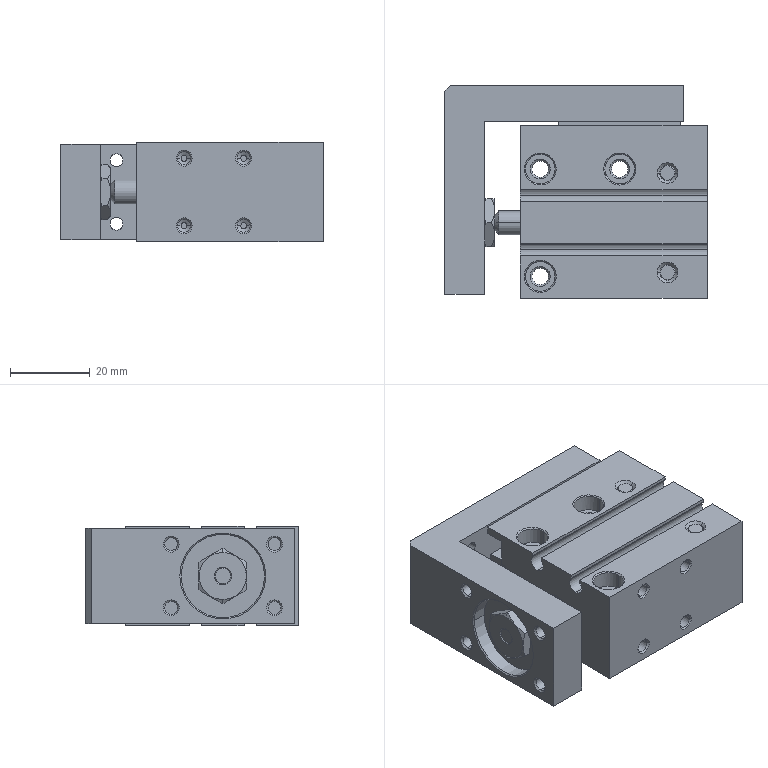Part | SolidWorks | 2 solids | 370 faces | box 66 x 53.5 x 25 mm | volume 64012 mm3 | cone 144 | plane 110 | cylinder 108 | spline 8 | commonest cylinder face diameters 3.242 x32 6 x12 7.5 x12 4.134 x10 0.4 x8 2.88 x8